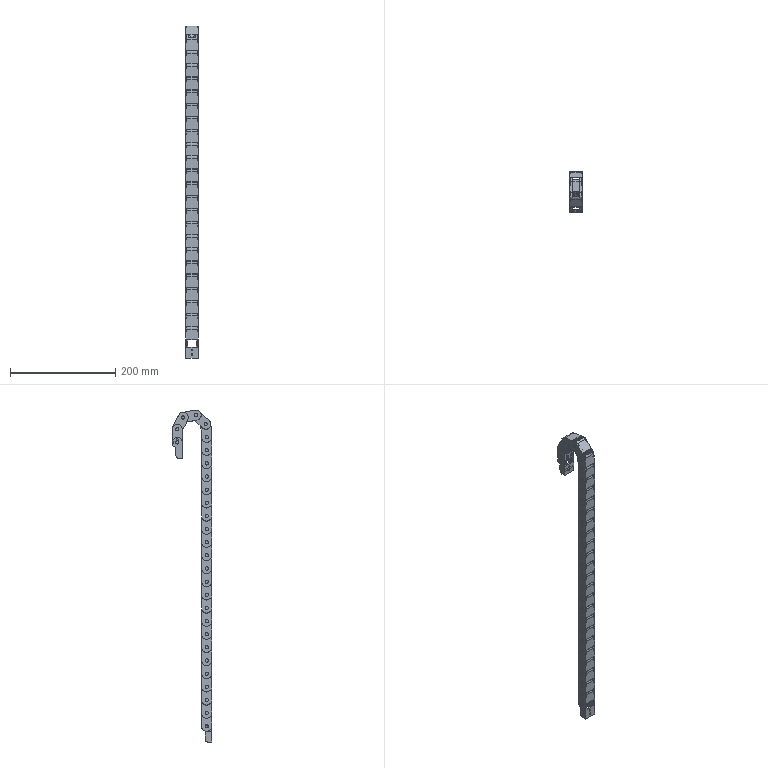Part | STEP file | 001-010-VBD02-F15-R28-N27 | 29 solids | 2510 faces | box 25.1 x 75.563 x 631.595 mm | volume 158989 mm3 | plane 1318 | cylinder 1180 | cone 8 | torus 4 | commonest cylinder face diameters 1 x270 6.1 x220 19.5 x189 2 x162 19.9 x135 2.4 x108